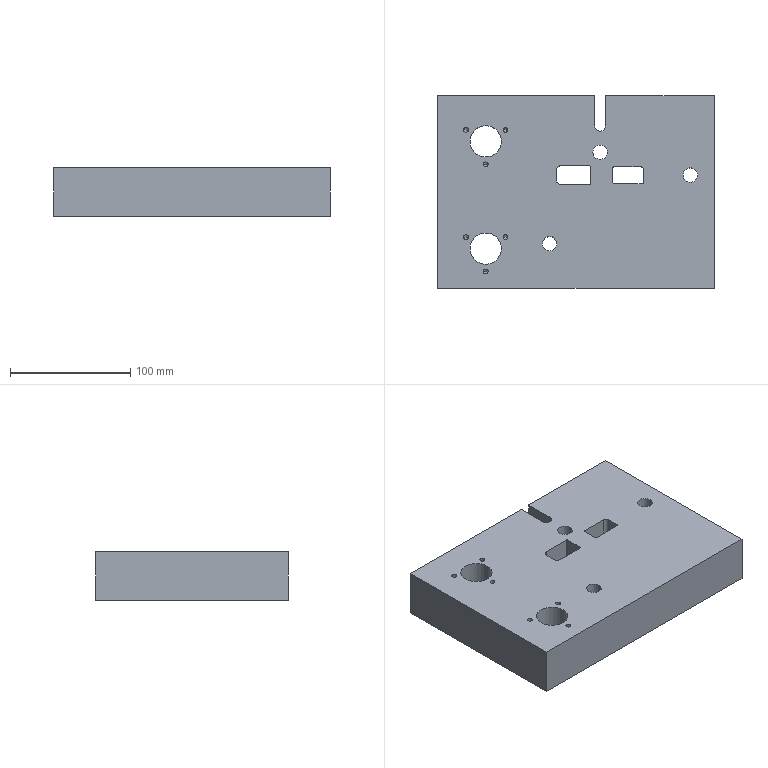Part | 1 solid | 87 faces | box 230 x 160 x 40 mm | volume 1292915 mm3 | cylinder 43 | plane 24 | cone 20 | commonest cylinder face diameters 4 x12 8 x10 12 x10 26 x4 3 x3 1 x2